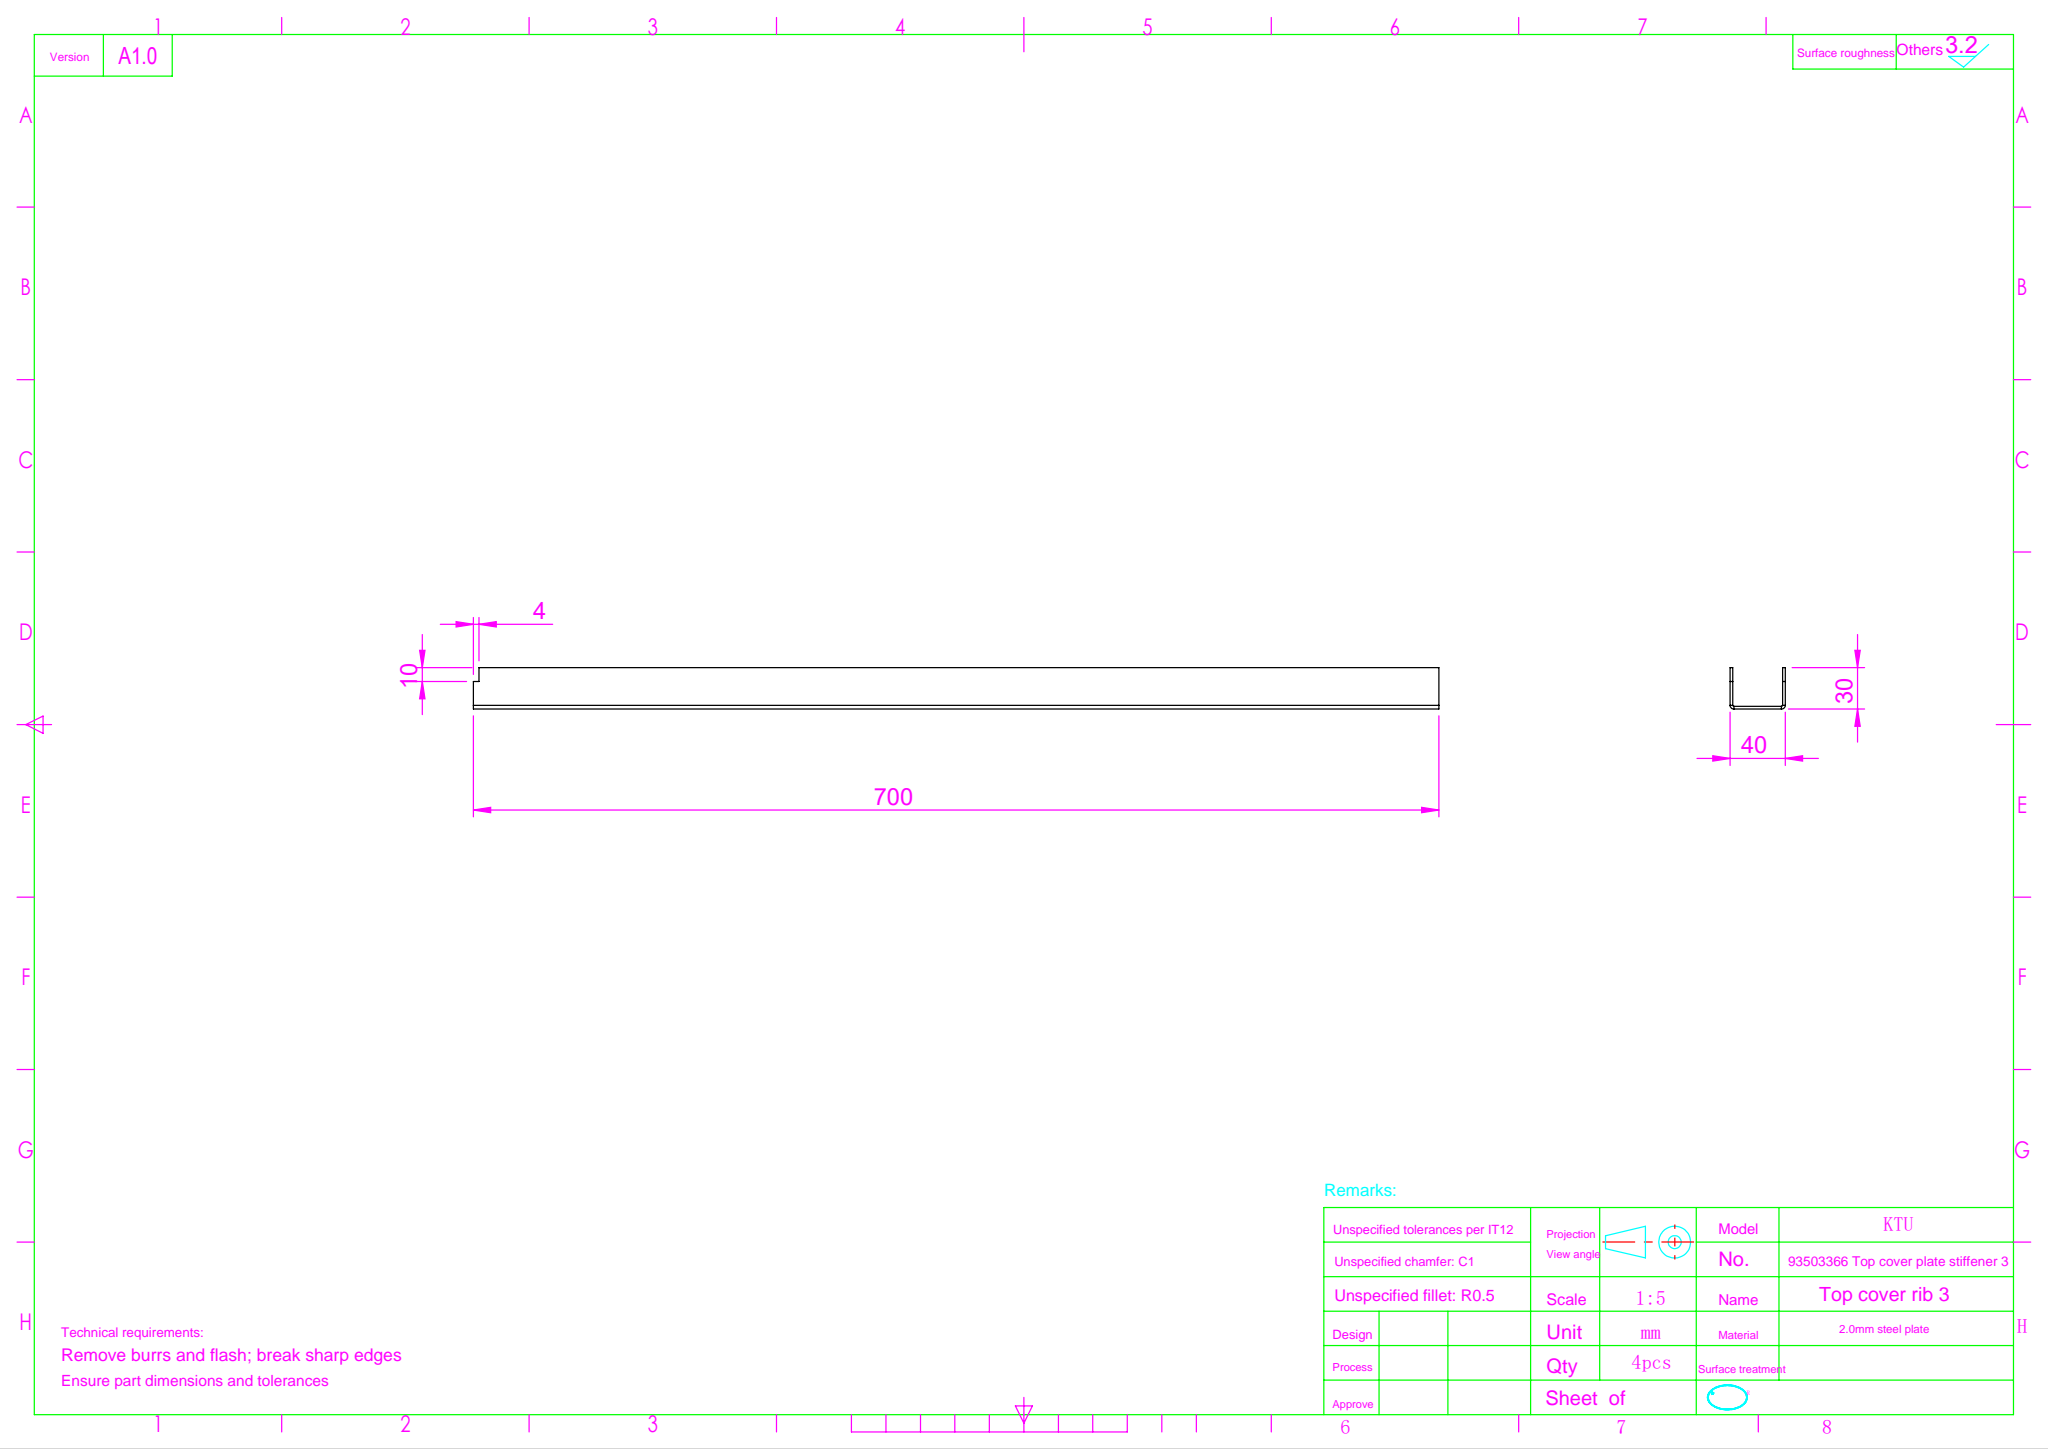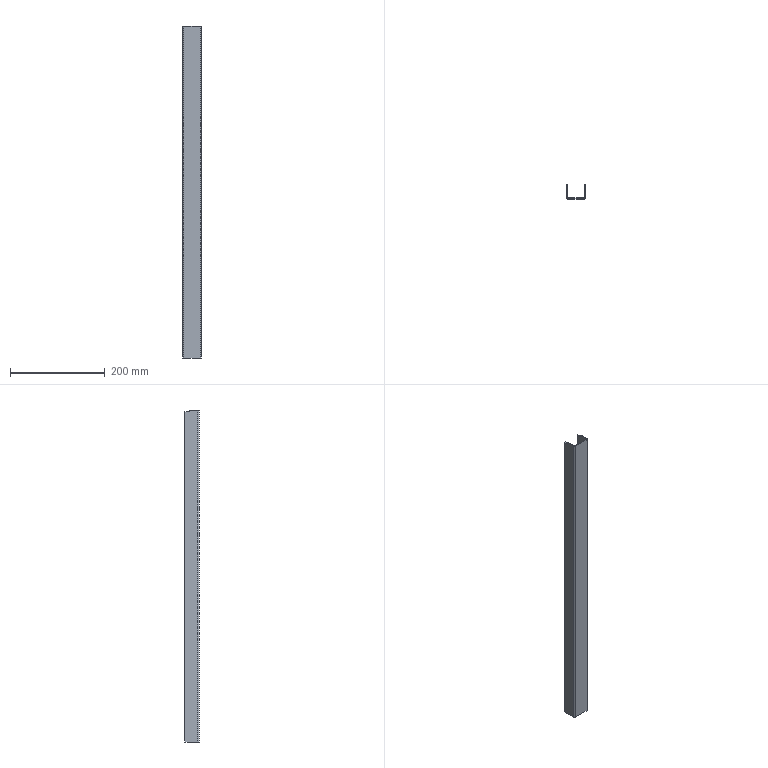Part | SolidWorks | features Cut 1, FlatPattern 1, SMBaseFlange 1, SheetMetal 1 | 1 solid | 26 faces | box 40 x 30 x 700 mm | volume 132153 mm3 | plane 22 | cylinder 4 | commonest cylinder face diameters 1.473 x2 5.473 x2
STEP:
#1=CARTESIAN_POINT('',(-20.,-12.263,350.));
#2=VERTEX_POINT('',#1);
#3=CARTESIAN_POINT('',(-18.,-12.263,350.));
#4=VERTEX_POINT('',#3);
#5=CARTESIAN_POINT('',(-20.,-12.263,350.));
#6=DIRECTION('',(1.,0.,0.));
#7=VECTOR('',#6,1000.);
#8=LINE('',#5,#7);
#9=EDGE_CURVE('',#2,#4,#8,.T.);
#10=ORIENTED_EDGE('',*,*,#9,.F.);
#11=CARTESIAN_POINT('',(-17.263,-15.,350.));
#12=VERTEX_POINT('',#11);
#13=CARTESIAN_POINT('',(-17.263,-12.263,350.));
#14=DIRECTION('',(0.,0.,1.));
#15=DIRECTION('',(-1.,0.,0.));
#16=AXIS2_PLACEMENT_3D('',#13,#14,#15);
#17=CIRCLE('',#16,2.737);
#18=EDGE_CURVE('',#2,#12,#17,.T.);
#19=ORIENTED_EDGE('',*,*,#18,.T.);
#20=CARTESIAN_POINT('',(-17.263,-13.,350.));
#21=VERTEX_POINT('',#20);
#22=CARTESIAN_POINT('',(-17.263,-13.,350.));
#23=DIRECTION('',(0.,-1.,0.));
#24=VECTOR('',#23,1000.);
#25=LINE('',#22,#24);
#26=EDGE_CURVE('',#21,#12,#25,.T.);
#27=ORIENTED_EDGE('',*,*,#26,.F.);
#28=CARTESIAN_POINT('',(-17.263,-12.263,350.));
#29=DIRECTION('',(0.,0.,1.));
#30=DIRECTION('',(1.,0.,0.));
#31=AXIS2_PLACEMENT_3D('',#28,#29,#30);
#32=CIRCLE('',#31,0.7366);
#33=EDGE_CURVE('',#4,#21,#32,.T.);
#34=ORIENTED_EDGE('',*,*,#33,.F.);
#35=EDGE_LOOP('',(#10,#19,#27,#34));
#36=FACE_OUTER_BOUND('',#35,.T.);
#37=CARTESIAN_POINT('',(-20.,-12.263,350.));
#38=DIRECTION('',(0.,0.,1.));
#39=DIRECTION('',(1.,0.,0.));
#40=AXIS2_PLACEMENT_3D('',#37,#38,#39);
#41=PLANE('',#40);
#42=ADVANCED_FACE('',(#36),#41,.T.);
#43=CARTESIAN_POINT('',(-20.,5.,350.));
#44=VERTEX_POINT('',#43);
#45=CARTESIAN_POINT('',(-18.,5.,350.));
#46=VERTEX_POINT('',#45);
#47=CARTESIAN_POINT('',(-20.,5.,350.));
#48=DIRECTION('',(1.,0.,0.));
#49=VECTOR('',#48,1000.);
#50=LINE('',#47,#49);
#51=EDGE_CURVE('',#44,#46,#50,.T.);
#52=ORIENTED_EDGE('',*,*,#51,.F.);
#53=CARTESIAN_POINT('',(-20.,-15.,350.));
#54=DIRECTION('',(0.,-1.,0.));
#55=VECTOR('',#54,1000.);
#56=LINE('',#53,#55);
#57=EDGE_CURVE('',#44,#2,#56,.T.);
#58=ORIENTED_EDGE('',*,*,#57,.T.);
#59=ORIENTED_EDGE('',*,*,#9,.T.);
#60=CARTESIAN_POINT('',(-18.,-15.,350.));
#61=DIRECTION('',(0.,-1.,0.));
#62=VECTOR('',#61,1000.);
#63=LINE('',#60,#62);
#64=EDGE_CURVE('',#46,#4,#63,.T.);
#65=ORIENTED_EDGE('',*,*,#64,.F.);
#66=EDGE_LOOP('',(#52,#58,#59,#65));
#67=FACE_OUTER_BOUND('',#66,.T.);
#68=CARTESIAN_POINT('',(-17.263,-13.,350.));
#69=DIRECTION('',(0.,0.,1.));
#70=DIRECTION('',(1.,0.,0.));
#71=AXIS2_PLACEMENT_3D('',#68,#69,#70);
#72=PLANE('',#71);
#73=ADVANCED_FACE('',(#67),#72,.T.);
#74=CARTESIAN_POINT('',(-17.263,-15.,-350.));
#75=VERTEX_POINT('',#74);
#76=CARTESIAN_POINT('',(-17.263,-13.,-350.));
#77=VERTEX_POINT('',#76);
#78=CARTESIAN_POINT('',(-17.263,-15.,-350.));
#79=DIRECTION('',(0.,1.,0.));
#80=VECTOR('',#79,1000.);
#81=LINE('',#78,#80);
#82=EDGE_CURVE('',#75,#77,#81,.T.);
#83=ORIENTED_EDGE('',*,*,#82,.F.);
#84=CARTESIAN_POINT('',(-20.,-12.263,-350.));
#85=VERTEX_POINT('',#84);
#86=CARTESIAN_POINT('',(-17.263,-12.263,-350.));
#87=DIRECTION('',(0.,0.,1.));
#88=DIRECTION('',(-1.,0.,0.));
#89=AXIS2_PLACEMENT_3D('',#86,#87,#88);
#90=CIRCLE('',#89,2.737);
#91=EDGE_CURVE('',#85,#75,#90,.T.);
#92=ORIENTED_EDGE('',*,*,#91,.F.);
#93=CARTESIAN_POINT('',(-18.,-12.263,-350.));
#94=VERTEX_POINT('',#93);
#95=CARTESIAN_POINT('',(-18.,-12.263,-350.));
#96=DIRECTION('',(-1.,0.,0.));
#97=VECTOR('',#96,1000.);
#98=LINE('',#95,#97);
#99=EDGE_CURVE('',#94,#85,#98,.T.);
#100=ORIENTED_EDGE('',*,*,#99,.F.);
#101=CARTESIAN_POINT('',(-17.263,-12.263,-350.));
#102=DIRECTION('',(0.,0.,1.));
#103=DIRECTION('',(1.,0.,0.));
#104=AXIS2_PLACEMENT_3D('',#101,#102,#103);
#105=CIRCLE('',#104,0.7366);
#106=EDGE_CURVE('',#94,#77,#105,.T.);
#107=ORIENTED_EDGE('',*,*,#106,.T.);
#108=EDGE_LOOP('',(#83,#92,#100,#107));
#109=FACE_OUTER_BOUND('',#108,.T.);
#110=CARTESIAN_POINT('',(-17.263,-15.,-350.));
#111=DIRECTION('',(0.,0.,-1.));
#112=DIRECTION('',(-1.,0.,0.));
#113=AXIS2_PLACEMENT_3D('',#110,#111,#112);
#114=PLANE('',#113);
#115=ADVANCED_FACE('',(#109),#114,.T.);
#116=CARTESIAN_POINT('',(17.263,-15.,-350.));
#117=VERTEX_POINT('',#116);
#118=CARTESIAN_POINT('',(20.,-15.,-350.));
#119=DIRECTION('',(1.,0.,0.));
#120=VECTOR('',#119,1000.);
#121=LINE('',#118,#120);
#122=EDGE_CURVE('',#75,#117,#121,.T.);
#123=ORIENTED_EDGE('',*,*,#122,.F.);
#124=ORIENTED_EDGE('',*,*,#82,.T.);
#125=CARTESIAN_POINT('',(17.263,-13.,-350.));
#126=VERTEX_POINT('',#125);
#127=CARTESIAN_POINT('',(20.,-13.,-350.));
#128=DIRECTION('',(1.,0.,0.));
#129=VECTOR('',#128,1000.);
#130=LINE('',#127,#129);
#131=EDGE_CURVE('',#77,#126,#130,.T.);
#132=ORIENTED_EDGE('',*,*,#131,.T.);
#133=CARTESIAN_POINT('',(17.263,-13.,-350.));
#134=DIRECTION('',(0.,-1.,0.));
#135=VECTOR('',#134,1000.);
#136=LINE('',#133,#135);
#137=EDGE_CURVE('',#126,#117,#136,.T.);
#138=ORIENTED_EDGE('',*,*,#137,.T.);
#139=EDGE_LOOP('',(#123,#124,#132,#138));
#140=FACE_OUTER_BOUND('',#139,.T.);
#141=CARTESIAN_POINT('',(-18.,-12.263,-350.));
#142=DIRECTION('',(0.,0.,-1.));
#143=DIRECTION('',(-1.,0.,0.));
#144=AXIS2_PLACEMENT_3D('',#141,#142,#143);
#145=PLANE('',#144);
#146=ADVANCED_FACE('',(#140),#145,.T.);
#147=CARTESIAN_POINT('',(17.263,-15.,350.));
#148=VERTEX_POINT('',#147);
#149=CARTESIAN_POINT('',(17.263,-13.,350.));
#150=VERTEX_POINT('',#149);
#151=CARTESIAN_POINT('',(17.263,-15.,350.));
#152=DIRECTION('',(0.,1.,0.));
#153=VECTOR('',#152,1000.);
#154=LINE('',#151,#153);
#155=EDGE_CURVE('',#148,#150,#154,.T.);
#156=ORIENTED_EDGE('',*,*,#155,.F.);
#157=CARTESIAN_POINT('',(20.,-12.263,350.));
#158=VERTEX_POINT('',#157);
#159=CARTESIAN_POINT('',(17.263,-12.263,350.));
#160=DIRECTION('',(0.,0.,1.));
#161=DIRECTION('',(-1.,0.,0.));
#162=AXIS2_PLACEMENT_3D('',#159,#160,#161);
#163=CIRCLE('',#162,2.737);
#164=EDGE_CURVE('',#148,#158,#163,.T.);
#165=ORIENTED_EDGE('',*,*,#164,.T.);
#166=CARTESIAN_POINT('',(18.,-12.263,350.));
#167=VERTEX_POINT('',#166);
#168=CARTESIAN_POINT('',(18.,-12.263,350.));
#169=DIRECTION('',(1.,0.,0.));
#170=VECTOR('',#169,1000.);
#171=LINE('',#168,#170);
#172=EDGE_CURVE('',#167,#158,#171,.T.);
#173=ORIENTED_EDGE('',*,*,#172,.F.);
#174=CARTESIAN_POINT('',(17.263,-12.263,350.));
#175=DIRECTION('',(0.,0.,1.));
#176=DIRECTION('',(1.,0.,0.));
#177=AXIS2_PLACEMENT_3D('',#174,#175,#176);
#178=CIRCLE('',#177,0.7366);
#179=EDGE_CURVE('',#150,#167,#178,.T.);
#180=ORIENTED_EDGE('',*,*,#179,.F.);
#181=EDGE_LOOP('',(#156,#165,#173,#180));
#182=FACE_OUTER_BOUND('',#181,.T.);
#183=CARTESIAN_POINT('',(17.263,-15.,350.));
#184=DIRECTION('',(0.,0.,1.));
#185=DIRECTION('',(1.,0.,0.));
#186=AXIS2_PLACEMENT_3D('',#183,#184,#185);
#187=PLANE('',#186);
#188=ADVANCED_FACE('',(#182),#187,.T.);
#189=CARTESIAN_POINT('',(20.,-15.,350.));
#190=DIRECTION('',(1.,0.,0.));
#191=VECTOR('',#190,1000.);
#192=LINE('',#189,#191);
#193=EDGE_CURVE('',#12,#148,#192,.T.);
#194=ORIENTED_EDGE('',*,*,#193,.T.);
#195=ORIENTED_EDGE('',*,*,#155,.T.);
#196=CARTESIAN_POINT('',(20.,-13.,350.));
#197=DIRECTION('',(1.,0.,0.));
#198=VECTOR('',#197,1000.);
#199=LINE('',#196,#198);
#200=EDGE_CURVE('',#21,#150,#199,.T.);
#201=ORIENTED_EDGE('',*,*,#200,.F.);
#202=ORIENTED_EDGE('',*,*,#26,.T.);
#203=EDGE_LOOP('',(#194,#195,#201,#202));
#204=FACE_OUTER_BOUND('',#203,.T.);
#205=CARTESIAN_POINT('',(18.,-12.263,350.));
#206=DIRECTION('',(0.,0.,1.));
#207=DIRECTION('',(1.,0.,0.));
#208=AXIS2_PLACEMENT_3D('',#205,#206,#207);
#209=PLANE('',#208);
#210=ADVANCED_FACE('',(#204),#209,.T.);
#211=CARTESIAN_POINT('',(20.,-12.263,-350.));
#212=VERTEX_POINT('',#211);
#213=CARTESIAN_POINT('',(18.,-12.263,-350.));
#214=VERTEX_POINT('',#213);
#215=CARTESIAN_POINT('',(20.,-12.263,-350.));
#216=DIRECTION('',(-1.,0.,0.));
#217=VECTOR('',#216,1000.);
#218=LINE('',#215,#217);
#219=EDGE_CURVE('',#212,#214,#218,.T.);
#220=ORIENTED_EDGE('',*,*,#219,.F.);
#221=CARTESIAN_POINT('',(17.263,-12.263,-350.));
#222=DIRECTION('',(0.,0.,1.));
#223=DIRECTION('',(-1.,0.,0.));
#224=AXIS2_PLACEMENT_3D('',#221,#222,#223);
#225=CIRCLE('',#224,2.737);
#226=EDGE_CURVE('',#117,#212,#225,.T.);
#227=ORIENTED_EDGE('',*,*,#226,.F.);
#228=ORIENTED_EDGE('',*,*,#137,.F.);
#229=CARTESIAN_POINT('',(17.263,-12.263,-350.));
#230=DIRECTION('',(0.,0.,1.));
#231=DIRECTION('',(1.,0.,0.));
#232=AXIS2_PLACEMENT_3D('',#229,#230,#231);
#233=CIRCLE('',#232,0.7366);
#234=EDGE_CURVE('',#126,#214,#233,.T.);
#235=ORIENTED_EDGE('',*,*,#234,.T.);
#236=EDGE_LOOP('',(#220,#227,#228,#235));
#237=FACE_OUTER_BOUND('',#236,.T.);
#238=CARTESIAN_POINT('',(20.,-12.263,-350.));
#239=DIRECTION('',(0.,0.,-1.));
#240=DIRECTION('',(-1.,0.,0.));
#241=AXIS2_PLACEMENT_3D('',#238,#239,#240);
#242=PLANE('',#241);
#243=ADVANCED_FACE('',(#237),#242,.T.);
#244=CARTESIAN_POINT('',(20.,15.,-350.));
#245=VERTEX_POINT('',#244);
#246=CARTESIAN_POINT('',(20.,-15.,-350.));
#247=DIRECTION('',(0.,1.,0.));
#248=VECTOR('',#247,1000.);
#249=LINE('',#246,#248);
#250=EDGE_CURVE('',#212,#245,#249,.T.);
#251=ORIENTED_EDGE('',*,*,#250,.F.);
#252=ORIENTED_EDGE('',*,*,#219,.T.);
#253=CARTESIAN_POINT('',(18.,15.,-350.));
#254=VERTEX_POINT('',#253);
#255=CARTESIAN_POINT('',(18.,-15.,-350.));
#256=DIRECTION('',(0.,1.,0.));
#257=VECTOR('',#256,1000.);
#258=LINE('',#255,#257);
#259=EDGE_CURVE('',#214,#254,#258,.T.);
#260=ORIENTED_EDGE('',*,*,#259,.T.);
#261=CARTESIAN_POINT('',(18.,15.,-350.));
#262=DIRECTION('',(1.,0.,0.));
#263=VECTOR('',#262,1000.);
#264=LINE('',#261,#263);
#265=EDGE_CURVE('',#254,#245,#264,.T.);
#266=ORIENTED_EDGE('',*,*,#265,.T.);
#267=EDGE_LOOP('',(#251,#252,#260,#266));
#268=FACE_OUTER_BOUND('',#267,.T.);
#269=CARTESIAN_POINT('',(17.263,-13.,-350.));
#270=DIRECTION('',(0.,0.,-1.));
#271=DIRECTION('',(-1.,0.,0.));
#272=AXIS2_PLACEMENT_3D('',#269,#270,#271);
#273=PLANE('',#272);
#274=ADVANCED_FACE('',(#268),#273,.T.);
#275=CARTESIAN_POINT('',(20.,15.,346.));
#276=VERTEX_POINT('',#275);
#277=CARTESIAN_POINT('',(20.,15.,350.));
#278=DIRECTION('',(0.,0.,-1.));
#279=VECTOR('',#278,1000.);
#280=LINE('',#277,#279);
#281=EDGE_CURVE('',#276,#245,#280,.T.);
#282=ORIENTED_EDGE('',*,*,#281,.F.);
#283=CARTESIAN_POINT('',(20.,5.,346.));
#284=VERTEX_POINT('',#283);
#285=CARTESIAN_POINT('',(20.,15.,346.));
#286=DIRECTION('',(0.,1.,0.));
#287=VECTOR('',#286,1000.);
#288=LINE('',#285,#287);
#289=EDGE_CURVE('',#284,#276,#288,.T.);
#290=ORIENTED_EDGE('',*,*,#289,.F.);
#291=CARTESIAN_POINT('',(20.,5.,350.));
#292=VERTEX_POINT('',#291);
#293=CARTESIAN_POINT('',(20.,5.,350.));
#294=DIRECTION('',(0.,0.,-1.));
#295=VECTOR('',#294,1000.);
#296=LINE('',#293,#295);
#297=EDGE_CURVE('',#292,#284,#296,.T.);
#298=ORIENTED_EDGE('',*,*,#297,.F.);
#299=CARTESIAN_POINT('',(20.,-15.,350.));
#300=DIRECTION('',(0.,1.,0.));
#301=VECTOR('',#300,1000.);
#302=LINE('',#299,#301);
#303=EDGE_CURVE('',#158,#292,#302,.T.);
#304=ORIENTED_EDGE('',*,*,#303,.F.);
#305=CARTESIAN_POINT('',(20.,-12.263,350.));
#306=DIRECTION('',(0.,0.,-1.));
#307=VECTOR('',#306,1000.);
#308=LINE('',#305,#307);
#309=EDGE_CURVE('',#158,#212,#308,.T.);
#310=ORIENTED_EDGE('',*,*,#309,.T.);
#311=ORIENTED_EDGE('',*,*,#250,.T.);
#312=EDGE_LOOP('',(#282,#290,#298,#304,#310,#311));
#313=FACE_OUTER_BOUND('',#312,.T.);
#314=CARTESIAN_POINT('',(20.,-15.,350.));
#315=DIRECTION('',(-1.,0.,0.));
#316=DIRECTION('',(0.,0.,1.));
#317=AXIS2_PLACEMENT_3D('',#314,#315,#316);
#318=PLANE('',#317);
#319=ADVANCED_FACE('',(#313),#318,.F.);
#320=CARTESIAN_POINT('',(18.,15.,346.));
#321=VERTEX_POINT('',#320);
#322=CARTESIAN_POINT('',(-20.,15.,346.));
#323=DIRECTION('',(1.,0.,0.));
#324=VECTOR('',#323,1000.);
#325=LINE('',#322,#324);
#326=EDGE_CURVE('',#321,#276,#325,.T.);
#327=ORIENTED_EDGE('',*,*,#326,.T.);
#328=ORIENTED_EDGE('',*,*,#281,.T.);
#329=ORIENTED_EDGE('',*,*,#265,.F.);
#330=CARTESIAN_POINT('',(18.,15.,350.));
#331=DIRECTION('',(0.,0.,-1.));
#332=VECTOR('',#331,1000.);
#333=LINE('',#330,#332);
#334=EDGE_CURVE('',#321,#254,#333,.T.);
#335=ORIENTED_EDGE('',*,*,#334,.F.);
#336=EDGE_LOOP('',(#327,#328,#329,#335));
#337=FACE_OUTER_BOUND('',#336,.T.);
#338=CARTESIAN_POINT('',(18.,15.,350.));
#339=DIRECTION('',(0.,1.,0.));
#340=DIRECTION('',(-1.,0.,0.));
#341=AXIS2_PLACEMENT_3D('',#338,#339,#340);
#342=PLANE('',#341);
#343=ADVANCED_FACE('',(#337),#342,.T.);
#344=CARTESIAN_POINT('',(18.,5.,346.));
#345=VERTEX_POINT('',#344);
#346=CARTESIAN_POINT('',(18.,-15.,346.));
#347=DIRECTION('',(0.,-1.,0.));
#348=VECTOR('',#347,1000.);
#349=LINE('',#346,#348);
#350=EDGE_CURVE('',#321,#345,#349,.T.);
#351=ORIENTED_EDGE('',*,*,#350,.F.);
#352=ORIENTED_EDGE('',*,*,#334,.T.);
#353=ORIENTED_EDGE('',*,*,#259,.F.);
#354=CARTESIAN_POINT('',(18.,-12.263,350.));
#355=DIRECTION('',(0.,0.,-1.));
#356=VECTOR('',#355,1000.);
#357=LINE('',#354,#356);
#358=EDGE_CURVE('',#167,#214,#357,.T.);
#359=ORIENTED_EDGE('',*,*,#358,.F.);
#360=CARTESIAN_POINT('',(18.,5.,350.));
#361=VERTEX_POINT('',#360);
#362=CARTESIAN_POINT('',(18.,-15.,350.));
#363=DIRECTION('',(0.,1.,0.));
#364=VECTOR('',#363,1000.);
#365=LINE('',#362,#364);
#366=EDGE_CURVE('',#167,#361,#365,.T.);
#367=ORIENTED_EDGE('',*,*,#366,.T.);
#368=CARTESIAN_POINT('',(18.,5.,350.));
#369=DIRECTION('',(0.,0.,1.));
#370=VECTOR('',#369,1000.);
#371=LINE('',#368,#370);
#372=EDGE_CURVE('',#345,#361,#371,.T.);
#373=ORIENTED_EDGE('',*,*,#372,.F.);
#374=EDGE_LOOP('',(#351,#352,#353,#359,#367,#373));
#375=FACE_OUTER_BOUND('',#374,.T.);
#376=CARTESIAN_POINT('',(18.,-15.,350.));
#377=DIRECTION('',(-1.,0.,0.));
#378=DIRECTION('',(0.,0.,1.));
#379=AXIS2_PLACEMENT_3D('',#376,#377,#378);
#380=PLANE('',#379);
#381=ADVANCED_FACE('',(#375),#380,.T.);
#382=ORIENTED_EDGE('',*,*,#234,.F.);
#383=CARTESIAN_POINT('',(17.263,-13.,350.));
#384=DIRECTION('',(0.,0.,-1.));
#385=VECTOR('',#384,1000.);
#386=LINE('',#383,#385);
#387=EDGE_CURVE('',#150,#126,#386,.T.);
#388=ORIENTED_EDGE('',*,*,#387,.F.);
#389=ORIENTED_EDGE('',*,*,#179,.T.);
#390=ORIENTED_EDGE('',*,*,#358,.T.);
#391=EDGE_LOOP('',(#382,#388,#389,#390));
#392=FACE_OUTER_BOUND('',#391,.T.);
#393=CARTESIAN_POINT('',(17.263,-12.263,350.));
#394=DIRECTION('',(0.,0.,-1.));
#395=DIRECTION('',(-1.,0.,0.));
#396=AXIS2_PLACEMENT_3D('',#393,#394,#395);
#397=CYLINDRICAL_SURFACE('',#396,0.7366);
#398=ADVANCED_FACE('',(#392),#397,.F.);
#399=ORIENTED_EDGE('',*,*,#131,.F.);
#400=CARTESIAN_POINT('',(-17.263,-13.,350.));
#401=DIRECTION('',(0.,0.,-1.));
#402=VECTOR('',#401,1000.);
#403=LINE('',#400,#402);
#404=EDGE_CURVE('',#21,#77,#403,.T.);
#405=ORIENTED_EDGE('',*,*,#404,.F.);
#406=ORIENTED_EDGE('',*,*,#200,.T.);
#407=ORIENTED_EDGE('',*,*,#387,.T.);
#408=EDGE_LOOP('',(#399,#405,#406,#407));
#409=FACE_OUTER_BOUND('',#408,.T.);
#410=CARTESIAN_POINT('',(20.,-13.,350.));
#411=DIRECTION('',(0.,1.,0.));
#412=DIRECTION('',(-1.,0.,0.));
#413=AXIS2_PLACEMENT_3D('',#410,#411,#412);
#414=PLANE('',#413);
#415=ADVANCED_FACE('',(#409),#414,.T.);
#416=ORIENTED_EDGE('',*,*,#106,.F.);
#417=CARTESIAN_POINT('',(-18.,-12.263,350.));
#418=DIRECTION('',(0.,0.,-1.));
#419=VECTOR('',#418,1000.);
#420=LINE('',#417,#419);
#421=EDGE_CURVE('',#4,#94,#420,.T.);
#422=ORIENTED_EDGE('',*,*,#421,.F.);
#423=ORIENTED_EDGE('',*,*,#33,.T.);
#424=ORIENTED_EDGE('',*,*,#404,.T.);
#425=EDGE_LOOP('',(#416,#422,#423,#424));
#426=FACE_OUTER_BOUND('',#425,.T.);
#427=CARTESIAN_POINT('',(-17.263,-12.263,350.));
#428=DIRECTION('',(0.,0.,-1.));
#429=DIRECTION('',(-1.,0.,0.));
#430=AXIS2_PLACEMENT_3D('',#427,#428,#429);
#431=CYLINDRICAL_SURFACE('',#430,0.7366);
#432=ADVANCED_FACE('',(#426),#431,.F.);
#433=CARTESIAN_POINT('',(-18.,5.,346.));
#434=VERTEX_POINT('',#433);
#435=CARTESIAN_POINT('',(-18.,15.,346.));
#436=VERTEX_POINT('',#435);
#437=CARTESIAN_POINT('',(-18.,-15.,346.));
#438=DIRECTION('',(0.,1.,0.));
#439=VECTOR('',#438,1000.);
#440=LINE('',#437,#439);
#441=EDGE_CURVE('',#434,#436,#440,.T.);
#442=ORIENTED_EDGE('',*,*,#441,.F.);
#443=CARTESIAN_POINT('',(-18.,5.,350.));
#444=DIRECTION('',(0.,0.,-1.));
#445=VECTOR('',#444,1000.);
#446=LINE('',#443,#445);
#447=EDGE_CURVE('',#46,#434,#446,.T.);
#448=ORIENTED_EDGE('',*,*,#447,.F.);
#449=ORIENTED_EDGE('',*,*,#64,.T.);
#450=ORIENTED_EDGE('',*,*,#421,.T.);
#451=CARTESIAN_POINT('',(-18.,15.,-350.));
#452=VERTEX_POINT('',#451);
#453=CARTESIAN_POINT('',(-18.,-15.,-350.));
#454=DIRECTION('',(0.,-1.,0.));
#455=VECTOR('',#454,1000.);
#456=LINE('',#453,#455);
#457=EDGE_CURVE('',#452,#94,#456,.T.);
#458=ORIENTED_EDGE('',*,*,#457,.F.);
#459=CARTESIAN_POINT('',(-18.,15.,350.));
#460=DIRECTION('',(0.,0.,-1.));
#461=VECTOR('',#460,1000.);
#462=LINE('',#459,#461);
#463=EDGE_CURVE('',#436,#452,#462,.T.);
#464=ORIENTED_EDGE('',*,*,#463,.F.);
#465=EDGE_LOOP('',(#442,#448,#449,#450,#458,#464));
#466=FACE_OUTER_BOUND('',#465,.T.);
#467=CARTESIAN_POINT('',(-18.,-15.,350.));
#468=DIRECTION('',(1.,0.,0.));
#469=DIRECTION('',(0.,0.,-1.));
#470=AXIS2_PLACEMENT_3D('',#467,#468,#469);
#471=PLANE('',#470);
#472=ADVANCED_FACE('',(#466),#471,.T.);
#473=CARTESIAN_POINT('',(-20.,15.,346.));
#474=VERTEX_POINT('',#473);
#475=CARTESIAN_POINT('',(-20.,15.,346.));
#476=DIRECTION('',(1.,0.,0.));
#477=VECTOR('',#476,1000.);
#478=LINE('',#475,#477);
#479=EDGE_CURVE('',#474,#436,#478,.T.);
#480=ORIENTED_EDGE('',*,*,#479,.T.);
#481=ORIENTED_EDGE('',*,*,#463,.T.);
#482=CARTESIAN_POINT('',(-20.,15.,-350.));
#483=VERTEX_POINT('',#482);
#484=CARTESIAN_POINT('',(-20.,15.,-350.));
#485=DIRECTION('',(1.,0.,0.));
#486=VECTOR('',#485,1000.);
#487=LINE('',#484,#486);
#488=EDGE_CURVE('',#483,#452,#487,.T.);
#489=ORIENTED_EDGE('',*,*,#488,.F.);
#490=CARTESIAN_POINT('',(-20.,15.,350.));
#491=DIRECTION('',(0.,0.,-1.));
#492=VECTOR('',#491,1000.);
#493=LINE('',#490,#492);
#494=EDGE_CURVE('',#474,#483,#493,.T.);
#495=ORIENTED_EDGE('',*,*,#494,.F.);
#496=EDGE_LOOP('',(#480,#481,#489,#495));
#497=FACE_OUTER_BOUND('',#496,.T.);
#498=CARTESIAN_POINT('',(-20.,15.,350.));
#499=DIRECTION('',(0.,1.,0.));
#500=DIRECTION('',(-1.,0.,0.));
#501=AXIS2_PLACEMENT_3D('',#498,#499,#500);
#502=PLANE('',#501);
#503=ADVANCED_FACE('',(#497),#502,.T.);
#504=CARTESIAN_POINT('',(-20.,5.,346.));
#505=VERTEX_POINT('',#504);
#506=CARTESIAN_POINT('',(-20.,5.,350.));
#507=DIRECTION('',(0.,0.,-1.));
#508=VECTOR('',#507,1000.);
#509=LINE('',#506,#508);
#510=EDGE_CURVE('',#44,#505,#509,.T.);
#511=ORIENTED_EDGE('',*,*,#510,.T.);
#512=CARTESIAN_POINT('',(-20.,15.,346.));
#513=DIRECTION('',(0.,1.,0.));
#514=VECTOR('',#513,1000.);
#515=LINE('',#512,#514);
#516=EDGE_CURVE('',#505,#474,#515,.T.);
#517=ORIENTED_EDGE('',*,*,#516,.T.);
#518=ORIENTED_EDGE('',*,*,#494,.T.);
#519=CARTESIAN_POINT('',(-20.,-15.,-350.));
#520=DIRECTION('',(0.,-1.,0.));
#521=VECTOR('',#520,1000.);
#522=LINE('',#519,#521);
#523=EDGE_CURVE('',#483,#85,#522,.T.);
#524=ORIENTED_EDGE('',*,*,#523,.T.);
#525=CARTESIAN_POINT('',(-20.,-12.263,350.));
#526=DIRECTION('',(0.,0.,-1.));
#527=VECTOR('',#526,1000.);
#528=LINE('',#525,#527);
#529=EDGE_CURVE('',#2,#85,#528,.T.);
#530=ORIENTED_EDGE('',*,*,#529,.F.);
#531=ORIENTED_EDGE('',*,*,#57,.F.);
#532=EDGE_LOOP('',(#511,#517,#518,#524,#530,#531));
#533=FACE_OUTER_BOUND('',#532,.T.);
#534=CARTESIAN_POINT('',(-20.,-15.,350.));
#535=DIRECTION('',(1.,0.,0.));
#536=DIRECTION('',(0.,0.,-1.));
#537=AXIS2_PLACEMENT_3D('',#534,#535,#536);
#538=PLANE('',#537);
#539=ADVANCED_FACE('',(#533),#538,.F.);
#540=ORIENTED_EDGE('',*,*,#91,.T.);
#541=CARTESIAN_POINT('',(-17.263,-15.,350.));
#542=DIRECTION('',(0.,0.,-1.));
#543=VECTOR('',#542,1000.);
#544=LINE('',#541,#543);
#545=EDGE_CURVE('',#12,#75,#544,.T.);
#546=ORIENTED_EDGE('',*,*,#545,.F.);
#547=ORIENTED_EDGE('',*,*,#18,.F.);
#548=ORIENTED_EDGE('',*,*,#529,.T.);
#549=EDGE_LOOP('',(#540,#546,#547,#548));
#550=FACE_OUTER_BOUND('',#549,.T.);
#551=CARTESIAN_POINT('',(-17.263,-12.263,350.));
#552=DIRECTION('',(0.,0.,-1.));
#553=DIRECTION('',(-1.,0.,0.));
#554=AXIS2_PLACEMENT_3D('',#551,#552,#553);
#555=CYLINDRICAL_SURFACE('',#554,2.737);
#556=ADVANCED_FACE('',(#550),#555,.T.);
#557=ORIENTED_EDGE('',*,*,#122,.T.);
#558=CARTESIAN_POINT('',(17.263,-15.,350.));
#559=DIRECTION('',(0.,0.,-1.));
#560=VECTOR('',#559,1000.);
#561=LINE('',#558,#560);
#562=EDGE_CURVE('',#148,#117,#561,.T.);
#563=ORIENTED_EDGE('',*,*,#562,.F.);
#564=ORIENTED_EDGE('',*,*,#193,.F.);
#565=ORIENTED_EDGE('',*,*,#545,.T.);
#566=EDGE_LOOP('',(#557,#563,#564,#565));
#567=FACE_OUTER_BOUND('',#566,.T.);
#568=CARTESIAN_POINT('',(20.,-15.,350.));
#569=DIRECTION('',(0.,1.,0.));
#570=DIRECTION('',(-1.,0.,0.));
#571=AXIS2_PLACEMENT_3D('',#568,#569,#570);
#572=PLANE('',#571);
#573=ADVANCED_FACE('',(#567),#572,.F.);
#574=ORIENTED_EDGE('',*,*,#226,.T.);
#575=ORIENTED_EDGE('',*,*,#309,.F.);
#576=ORIENTED_EDGE('',*,*,#164,.F.);
#577=ORIENTED_EDGE('',*,*,#562,.T.);
#578=EDGE_LOOP('',(#574,#575,#576,#577));
#579=FACE_OUTER_BOUND('',#578,.T.);
#580=CARTESIAN_POINT('',(17.263,-12.263,350.));
#581=DIRECTION('',(0.,0.,-1.));
#582=DIRECTION('',(-1.,0.,0.));
#583=AXIS2_PLACEMENT_3D('',#580,#581,#582);
#584=CYLINDRICAL_SURFACE('',#583,2.737);
#585=ADVANCED_FACE('',(#579),#584,.T.);
#586=CARTESIAN_POINT('',(17.263,5.,350.));
#587=DIRECTION('',(1.,0.,0.));
#588=VECTOR('',#587,1000.);
#589=LINE('',#586,#588);
#590=EDGE_CURVE('',#361,#292,#589,.T.);
#591=ORIENTED_EDGE('',*,*,#590,.F.);
#592=ORIENTED_EDGE('',*,*,#366,.F.);
#593=ORIENTED_EDGE('',*,*,#172,.T.);
#594=ORIENTED_EDGE('',*,*,#303,.T.);
#595=EDGE_LOOP('',(#591,#592,#593,#594));
#596=FACE_OUTER_BOUND('',#595,.T.);
#597=CARTESIAN_POINT('',(17.263,-12.263,350.));
#598=DIRECTION('',(0.,0.,1.));
#599=DIRECTION('',(1.,0.,0.));
#600=AXIS2_PLACEMENT_3D('',#597,#598,#599);
#601=PLANE('',#600);
#602=ADVANCED_FACE('',(#596),#601,.T.);
#603=ORIENTED_EDGE('',*,*,#457,.T.);
#604=ORIENTED_EDGE('',*,*,#99,.T.);
#605=ORIENTED_EDGE('',*,*,#523,.F.);
#606=ORIENTED_EDGE('',*,*,#488,.T.);
#607=EDGE_LOOP('',(#603,#604,#605,#606));
#608=FACE_OUTER_BOUND('',#607,.T.);
#609=CARTESIAN_POINT('',(17.263,-12.263,-350.));
#610=DIRECTION('',(0.,0.,1.));
#611=DIRECTION('',(1.,0.,0.));
#612=AXIS2_PLACEMENT_3D('',#609,#610,#611);
#613=PLANE('',#612);
#614=ADVANCED_FACE('',(#608),#613,.F.);
#615=ORIENTED_EDGE('',*,*,#372,.T.);
#616=ORIENTED_EDGE('',*,*,#590,.T.);
#617=ORIENTED_EDGE('',*,*,#297,.T.);
#618=CARTESIAN_POINT('',(-20.,5.,346.));
#619=DIRECTION('',(1.,0.,0.));
#620=VECTOR('',#619,1000.);
#621=LINE('',#618,#620);
#622=EDGE_CURVE('',#345,#284,#621,.T.);
#623=ORIENTED_EDGE('',*,*,#622,.F.);
#624=EDGE_LOOP('',(#615,#616,#617,#623));
#625=FACE_OUTER_BOUND('',#624,.T.);
#626=CARTESIAN_POINT('',(-20.,5.,350.));
#627=DIRECTION('',(0.,-1.,0.));
#628=DIRECTION('',(0.,0.,-1.));
#629=AXIS2_PLACEMENT_3D('',#626,#627,#628);
#630=PLANE('',#629);
#631=ADVANCED_FACE('',(#625),#630,.F.);
#632=ORIENTED_EDGE('',*,*,#350,.T.);
#633=ORIENTED_EDGE('',*,*,#622,.T.);
#634=ORIENTED_EDGE('',*,*,#289,.T.);
#635=ORIENTED_EDGE('',*,*,#326,.F.);
#636=EDGE_LOOP('',(#632,#633,#634,#635));
#637=FACE_OUTER_BOUND('',#636,.T.);
#638=CARTESIAN_POINT('',(-20.,15.,346.));
#639=DIRECTION('',(0.,0.,-1.));
#640=DIRECTION('',(-1.,0.,0.));
#641=AXIS2_PLACEMENT_3D('',#638,#639,#640);
#642=PLANE('',#641);
#643=ADVANCED_FACE('',(#637),#642,.F.);
#644=ORIENTED_EDGE('',*,*,#441,.T.);
#645=ORIENTED_EDGE('',*,*,#479,.F.);
#646=ORIENTED_EDGE('',*,*,#516,.F.);
#647=CARTESIAN_POINT('',(-20.,5.,346.));
#648=DIRECTION('',(1.,0.,0.));
#649=VECTOR('',#648,1000.);
#650=LINE('',#647,#649);
#651=EDGE_CURVE('',#505,#434,#650,.T.);
#652=ORIENTED_EDGE('',*,*,#651,.T.);
#653=EDGE_LOOP('',(#644,#645,#646,#652));
#654=FACE_OUTER_BOUND('',#653,.T.);
#655=CARTESIAN_POINT('',(-20.,15.,346.));
#656=DIRECTION('',(0.,0.,-1.));
#657=DIRECTION('',(-1.,0.,0.));
#658=AXIS2_PLACEMENT_3D('',#655,#656,#657);
#659=PLANE('',#658);
#660=ADVANCED_FACE('',(#654),#659,.F.);
#661=ORIENTED_EDGE('',*,*,#447,.T.);
#662=ORIENTED_EDGE('',*,*,#651,.F.);
#663=ORIENTED_EDGE('',*,*,#510,.F.);
#664=ORIENTED_EDGE('',*,*,#51,.T.);
#665=EDGE_LOOP('',(#661,#662,#663,#664));
#666=FACE_OUTER_BOUND('',#665,.T.);
#667=CARTESIAN_POINT('',(-20.,5.,350.));
#668=DIRECTION('',(0.,-1.,0.));
#669=DIRECTION('',(0.,0.,-1.));
#670=AXIS2_PLACEMENT_3D('',#667,#668,#669);
#671=PLANE('',#670);
#672=ADVANCED_FACE('',(#666),#671,.F.);
#673=CLOSED_SHELL('',(#42,#73,#115,#146,#188,#210,#243,#274,#319,#343,#381,#398,#415,#432,#472,#503,#539,#556,#573,#585,#602,#614,#631,#643,#660,#672));
#674=MANIFOLD_SOLID_BREP('',#673);
#675=CARTESIAN_POINT('',(0.,0.,0.));
#676=DIRECTION('',(0.,0.,1.));
#677=DIRECTION('',(1.,0.,0.));
#678=AXIS2_PLACEMENT_3D('',#675,#676,#677);
#679=(LENGTH_UNIT()NAMED_UNIT(*)SI_UNIT(.MILLI.,.METRE.));
#680=UNCERTAINTY_MEASURE_WITH_UNIT(LENGTH_MEASURE(0.00001),#679,'','');
#681=(NAMED_UNIT(*)PLANE_ANGLE_UNIT()SI_UNIT($,.RADIAN.));
#682=(NAMED_UNIT(*)SI_UNIT($,.STERADIAN.)SOLID_ANGLE_UNIT());
#683=(GEOMETRIC_REPRESENTATION_CONTEXT(3)GLOBAL_UNCERTAINTY_ASSIGNED_CONTEXT((#680))GLOBAL_UNIT_ASSIGNED_CONTEXT((#679,#681,#682))REPRESENTATION_CONTEXT('',''));
#684=ADVANCED_BREP_SHAPE_REPRESENTATION('',(#674,#678),#683);